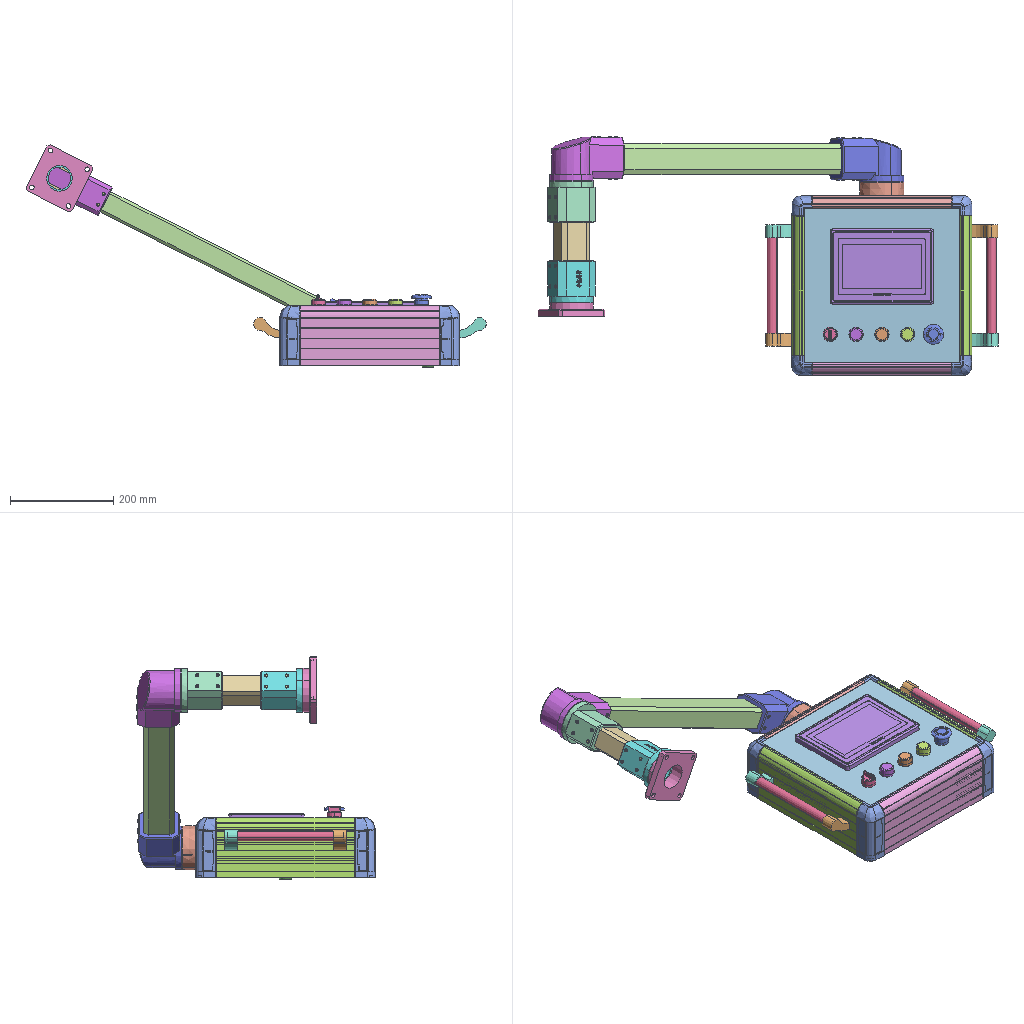Assembly | SolidWorks | 31 different items | 63 placed | box 892 x 463 x 431 mm
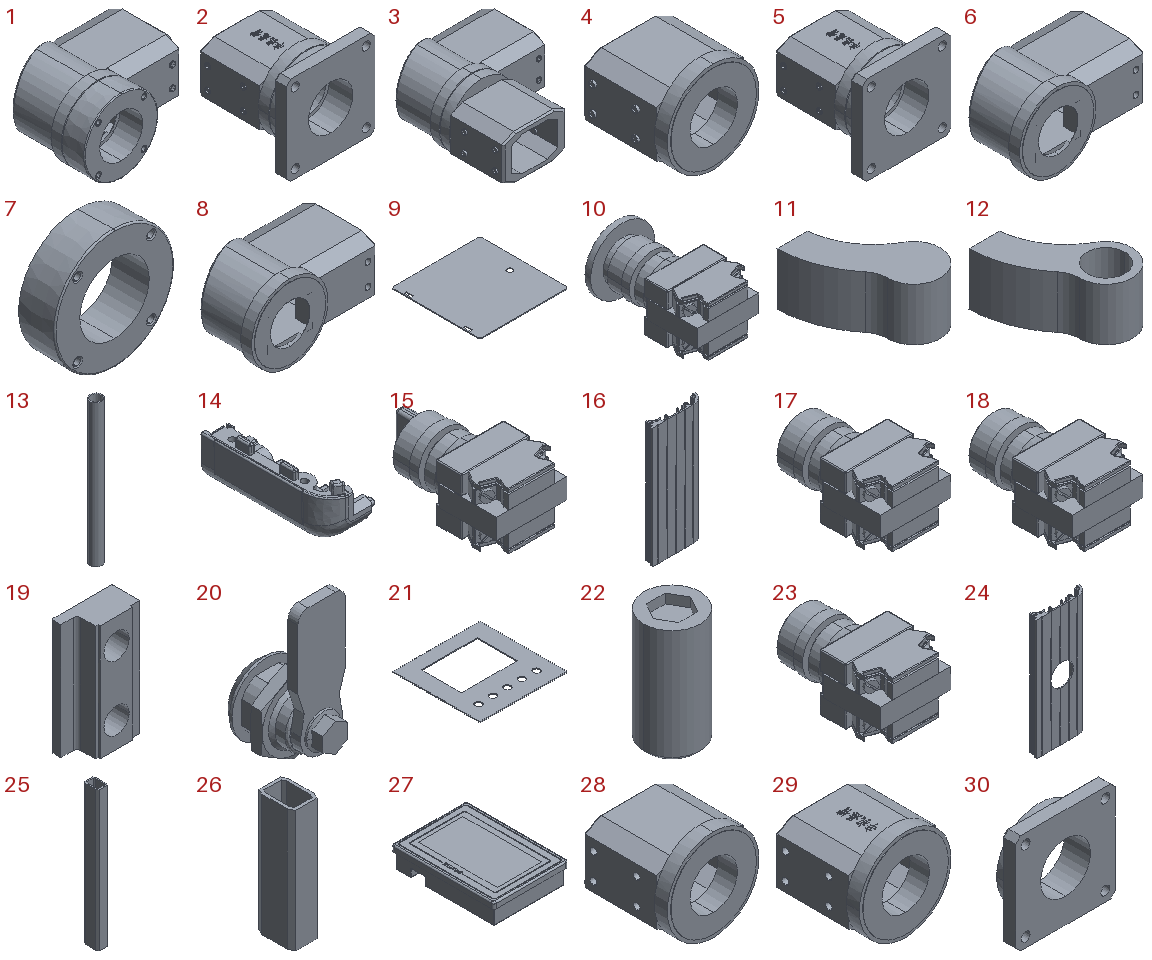Parts list (item | name | quantity | parent item | size | volume | features):
1 | (subassembly) | x1 | - | 142.981 x 112.5 x 85.962 mm | 471126 mm3 | -
2 | (subassembly) | x1 | in 5 | 100 x 108 x 100 mm | 341728 mm3 | -
3 | (subassembly) | x1 | - | 142.662 x 167.109 x 85 mm | 575306 mm3 | -
4 | (subassembly) | x1 | in 3 | 85.162 x 81 x 85 mm | 190340 mm3 | features CompositeCurve 1
5 | (subassembly) | x1 | - | 100 x 108 x 100 mm | 341728 mm3 | -
6 | - | x1 | in 3 | 142.5 x 84.5 x 85 mm | 382964 mm3 | features BaseBody 1
7 | - | x1 | in 1 | 85.962 x 26.5 x 85.962 mm | 97958 mm3 | features BaseBody 1
8 | - | x1 | in 1 | 142.5 x 84.5 x 85 mm | 371166 mm3 | features BaseBody 1
9 | - | x1 | - | 336 x 336 x 3 mm | 335960 mm3 | features Extrusion 1, ICE 1
10 | - | x1 | - | 39 x 70 x 39 mm | 55786 mm3 | features BaseBody 3
11 | - | x2 | - | 39.25 x 51 x 25 mm | 19641 mm3 | features BaseBody 1
12 | - | x2 | - | 39.25 x 51 x 25 mm | 19641 mm3 | features BaseBody 1
13 | - | x2 | - | 19 x 19 x 225 mm | 18555 mm3 | features BaseBody 1
14 | - | x4 | - | 46.838 x 116.267 x 46.838 mm | 58227 mm3 | features BaseBody 1, ICE 1
15 | - | x1 | - | 37.364 x 70 x 30 mm | 49458 mm3 | features BaseBody 3, Fillet 2, ICE 2
16 | - | x1 | - | 116.267 x 23.727 x 270 mm | 211273 mm3 | features BaseBody 1
17 | - | x1 | - | 37.364 x 62 x 30 mm | 48495 mm3 | features BaseBody 3, Fillet 1, ICE 1
18 | - | x1 | - | 37.364 x 62 x 30 mm | 48495 mm3 | features BaseBody 3, Fillet 1, ICE 1
19 | - | x2 | - | 13.1 x 6.5 x 25 mm | 1279 mm3 | features BaseBody 1
20 | - | x1 | - | 28 x 32 x 60.591 mm | 13256 mm3 | features BaseBody 1
21 | - | x1 | - | 300 x 300 x 3 mm | 184548 mm3 | features BaseBody 1
22 | - | x25 | in 1, 2, 3, 4 | 6 x 6 x 12.25 mm | 333.743 mm3 | features BaseBody 1
23 | - | x1 | - | 37.364 x 62 x 30 mm | 48495 mm3 | features BaseBody 3, Fillet 1, ICE 1
24 | - | x1 | - | 116.267 x 23.727 x 270 mm | 194333 mm3 | features BaseBody 1
25 | - | x1 | - | 44 x 60.7 x 600 mm | 534048 mm3 | features Extrusion 1
26 | - | x1 | - | 44 x 60.7 x 200 mm | 178016 mm3 | features Extrusion 1
27 | - | x1 | - | 146.35 x 200.35 x 42.55 mm | 1144321 mm3 | features ICE 7, Fillet 3, Extrusion 1
28 | - | x1 | in 4 | 85 x 81 x 85 mm | 188004 mm3 | features BaseBody 1
29 | - | x1 | in 2 | 85 x 81 x 85 mm | 187992 mm3 | features BaseBody 1
30 | - | x1 | in 2 | 100 x 26.5 x 100 mm | 151734 mm3 | features BaseBody 1
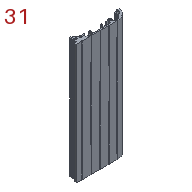31 | - | x2 | - | 116.267 x 23.727 x 270 mm | 211273 mm3 | features BaseBody 1
Mates (type | each side: item.copy, entity, surface, feature):
In the top assembly
Coincident | 8.1 face plane Input1 | 25.1 face plane Boss-Extrude1 | 3 times
Coincident | 6.1 face plane Input1 | 25.1 face plane Boss-Extrude1 | 2 times
Coincident | 28.1 face plane Input1 | 29.1 face plane Input1 | 3 times
Coincident | 28.1 face plane Input1 | 26.1 face plane Boss-Extrude1 | 3 times
Coincident | 29.1 face plane Input1 | 26.1 face plane Boss-Extrude1
Coincident | 21.1 face plane Input1 | 27.1 face plane Extrude2 | 2 times
Coincident | 21.1 face plane Input1 | 27.1 face plane Extrude1
Parallel | 24.1 face plane Input1 | 20.1 face plane Input1
Concentric | 20.1 face cylinder Input1 | 9.1 face cylinder Boss-Extrude1
Coincident | 20.1 face plane Input1 | 9.1 face plane Boss-Extrude1
Coincident | 14.1 face plane Input1 | 14.2 face plane Input1
Coincident | 16.1 face plane Input1 | 14.2 face plane Input1
Coincident | 31.1 face plane Input1 | 14.2 face plane Input1
Coincident | 16.1 face plane Input1 | 14.2 edge
Coincident | 24.1 face plane Input1 | 14.3 face plane Input1
Coincident | 31.2 face plane Input1 | 14.3 face plane Input1
Coincident | 14.2 face plane Input1 | 14.4 face plane Input1
Coincident | 16.1 face plane Input1 | 14.4 face plane Input1
Coincident | 31.2 face plane Input1 | 14.4 face plane Input1
Coincident | 31.2 face plane Input1 | 14.3 edge
Coincident | 14.1 face plane Input1 | 14.3 face plane Input1
Coincident | 13.1 edge | 12.1 face plane Input1
Coincident | 31.1 face plane Input1 | 12.1 face plane Input1
Concentric | 13.1 face cylinder Input1 | 12.1 face cylinder Input1
Coincident | 13.1 face plane Input1 | 11.1 face plane Input1
Coincident | 31.1 face plane Input1 | 11.1 face plane Input1
Concentric | 13.1 face cylinder Input1 | 11.1 face cylinder Input1
Coincident | 23.1 face plane Cut-Extrude1 | 18.1 face plane Cut-Extrude1
Coincident | 15.1 face plane Cut-Extrude1 | 18.1 face plane Cut-Extrude1
Coincident | 17.1 face plane Cut-Extrude1 | 23.1 face plane Cut-Extrude1
Coincident | 23.1 face plane Input3 | 10.1 face plane Input3
Coincident | 21.1 face plane Input1 | 23.1 face plane Input3
Concentric | 21.1 edge | 15.1 edge
Concentric | 21.1 edge | 18.1 face cylinder Input3
Concentric | 21.1 edge | 23.1 face cylinder Input3
Concentric | 21.1 edge | 17.1 face cylinder Input3
Concentric | 21.1 edge | 10.1 face cylinder Input3
Coincident | 17.1 face plane Input2 | 10.1 edge
In subassembly 2
Concentric | 22.1 face cylinder Input1 | 29.2 face cylinder Input1
Concentric | 22.2 face cylinder Input1 | 29.2 face cylinder Input1
Concentric | 22.3 face cylinder Input1 | 29.2 face cylinder Input1
Concentric | 22.4 face cylinder Input1 | 29.2 face cylinder Input1
Coincident | 22.4 face plane Input1 | 29.2 face plane Input1
In subassembly 3
Coincident | 6.2 face plane Input1 | 28.2 face plane Input1
Concentric | 6.2 face cylinder Input1 | 28.2 face cylinder Input1
Concentric | 6.2 face cylinder Input1 | 22.4 face cylinder Input1
Concentric | 6.2 face cylinder Input1 | 22.3 face cylinder Input1
Concentric | 6.2 face cylinder Input1 | 22.1 face cylinder Input1
Concentric | 6.2 face cylinder Input1 | 22.5 face cylinder Input1
Concentric | 22.2 face cylinder Input1 | 6.2 face cylinder Input1
Concentric | 6.2 face cylinder Input1 | 22.6 face cylinder Input1
In subassembly 4
Concentric | 22.5 face cylinder Input1 | 28.3 face cylinder Input1
Concentric | 22.1 face cylinder Input1 | 28.3 face cylinder Input1
Concentric | 28.3 face cylinder Input1 | 22.6 face cylinder Input1
Concentric | 22.2 edge | 28.3 face cylinder Input1
Concentric | 28.3 face cylinder Input1 | 22.7 face cylinder Input1
DistanceDim | 22.4 face plane Input1 | 28.3 face plane Input1
Coincident | 22.4 face plane Input1 | 22.7 face plane Input1